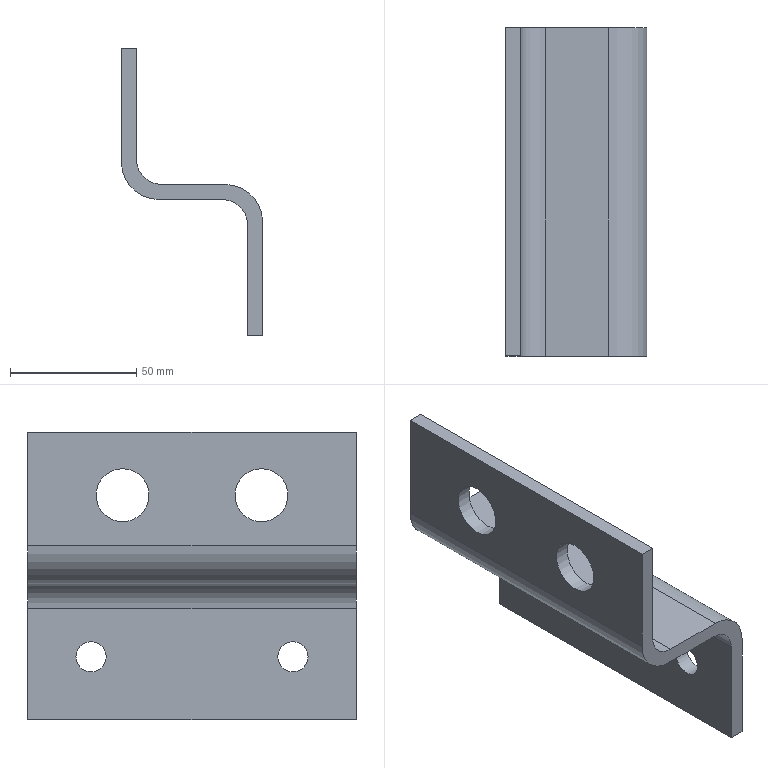Part | NX | features solid 2 | 1 solid | 18 faces | box 56 x 130 x 114 mm | volume 115432 mm3 | plane 10 | cylinder 8 | commonest cylinder face diameters 12 x2 20 x2 21 x2 30 x2
STEP:
#1=CARTESIAN_POINT('',(1315.,-200.,-620.));
#2=VERTEX_POINT('',#1);
#3=CARTESIAN_POINT('',(1321.,-200.,-620.));
#4=VERTEX_POINT('',#3);
#5=CARTESIAN_POINT('',(1325.,-200.,-620.));
#6=DIRECTION('',(-1.,0.,0.));
#7=VECTOR('',#6,1000.);
#8=LINE('',#5,#7);
#9=EDGE_CURVE('',#2,#4,#8,.F.);
#10=ORIENTED_EDGE('',*,*,#9,.T.);
#11=CARTESIAN_POINT('',(1321.,-330.,-620.));
#12=VERTEX_POINT('',#11);
#13=CARTESIAN_POINT('',(1321.,-130.,-620.));
#14=DIRECTION('',(0.,1.,0.));
#15=VECTOR('',#14,1000.);
#16=LINE('',#13,#15);
#17=EDGE_CURVE('',#4,#12,#16,.F.);
#18=ORIENTED_EDGE('',*,*,#17,.T.);
#19=CARTESIAN_POINT('',(1315.,-330.,-620.));
#20=VERTEX_POINT('',#19);
#21=CARTESIAN_POINT('',(1315.,-330.,-620.));
#22=DIRECTION('',(1.,0.,0.));
#23=VECTOR('',#22,1000.);
#24=LINE('',#21,#23);
#25=EDGE_CURVE('',#20,#12,#24,.T.);
#26=ORIENTED_EDGE('',*,*,#25,.F.);
#27=CARTESIAN_POINT('',(1315.,-130.,-620.));
#28=DIRECTION('',(0.,1.,0.));
#29=VECTOR('',#28,1000.);
#30=LINE('',#27,#29);
#31=EDGE_CURVE('',#2,#20,#30,.F.);
#32=ORIENTED_EDGE('',*,*,#31,.F.);
#33=EDGE_LOOP('',(#10,#18,#26,#32));
#34=FACE_BOUND('',#33,.T.);
#35=CARTESIAN_POINT('',(1325.,-130.,-620.));
#36=DIRECTION('',(0.,0.,-1.));
#37=DIRECTION('',(-1.,0.,0.));
#38=AXIS2_PLACEMENT_3D('',#35,#36,#37);
#39=PLANE('',#38);
#40=ADVANCED_FACE('',(#34),#39,.T.);
#41=CARTESIAN_POINT('',(1321.,-330.,-575.));
#42=VERTEX_POINT('',#41);
#43=CARTESIAN_POINT('',(1321.,-330.,-610.));
#44=DIRECTION('',(0.,0.,1.));
#45=VECTOR('',#44,1000.);
#46=LINE('',#43,#45);
#47=EDGE_CURVE('',#12,#42,#46,.T.);
#48=ORIENTED_EDGE('',*,*,#47,.T.);
#49=CARTESIAN_POINT('',(1306.,-330.,-560.));
#50=VERTEX_POINT('',#49);
#51=CARTESIAN_POINT('',(1306.,-330.,-575.));
#52=DIRECTION('',(0.,-1.,0.));
#53=DIRECTION('',(1.,0.,0.));
#54=AXIS2_PLACEMENT_3D('',#51,#52,#53);
#55=CIRCLE('',#54,15.);
#56=EDGE_CURVE('',#42,#50,#55,.T.);
#57=ORIENTED_EDGE('',*,*,#56,.T.);
#58=CARTESIAN_POINT('',(1281.,-330.,-560.));
#59=VERTEX_POINT('',#58);
#60=CARTESIAN_POINT('',(1315.,-330.,-560.));
#61=DIRECTION('',(-1.,0.,0.));
#62=VECTOR('',#61,1000.);
#63=LINE('',#60,#62);
#64=EDGE_CURVE('',#59,#50,#63,.F.);
#65=ORIENTED_EDGE('',*,*,#64,.F.);
#66=CARTESIAN_POINT('',(1271.,-330.,-550.));
#67=VERTEX_POINT('',#66);
#68=CARTESIAN_POINT('',(1281.,-330.,-550.));
#69=DIRECTION('',(0.,-1.,0.));
#70=DIRECTION('',(1.,0.,0.));
#71=AXIS2_PLACEMENT_3D('',#68,#69,#70);
#72=CIRCLE('',#71,10.);
#73=EDGE_CURVE('',#59,#67,#72,.F.);
#74=ORIENTED_EDGE('',*,*,#73,.T.);
#75=CARTESIAN_POINT('',(1271.,-330.,-506.));
#76=VERTEX_POINT('',#75);
#77=CARTESIAN_POINT('',(1271.,-330.,-504.5));
#78=DIRECTION('',(0.,0.,1.));
#79=VECTOR('',#78,1000.);
#80=LINE('',#77,#79);
#81=EDGE_CURVE('',#76,#67,#80,.F.);
#82=ORIENTED_EDGE('',*,*,#81,.F.);
#83=CARTESIAN_POINT('',(1265.,-330.,-506.));
#84=VERTEX_POINT('',#83);
#85=CARTESIAN_POINT('',(1267.,-330.,-506.));
#86=DIRECTION('',(-1.,0.,0.));
#87=VECTOR('',#86,1000.);
#88=LINE('',#85,#87);
#89=EDGE_CURVE('',#76,#84,#88,.T.);
#90=ORIENTED_EDGE('',*,*,#89,.T.);
#91=CARTESIAN_POINT('',(1265.,-330.,-551.));
#92=VERTEX_POINT('',#91);
#93=CARTESIAN_POINT('',(1265.,-330.,-555.5));
#94=DIRECTION('',(0.,0.,1.));
#95=VECTOR('',#94,1000.);
#96=LINE('',#93,#95);
#97=EDGE_CURVE('',#84,#92,#96,.F.);
#98=ORIENTED_EDGE('',*,*,#97,.T.);
#99=CARTESIAN_POINT('',(1280.,-330.,-566.));
#100=VERTEX_POINT('',#99);
#101=CARTESIAN_POINT('',(1280.,-330.,-551.));
#102=DIRECTION('',(0.,-1.,0.));
#103=DIRECTION('',(1.,0.,0.));
#104=AXIS2_PLACEMENT_3D('',#101,#102,#103);
#105=CIRCLE('',#104,15.);
#106=EDGE_CURVE('',#92,#100,#105,.T.);
#107=ORIENTED_EDGE('',*,*,#106,.T.);
#108=CARTESIAN_POINT('',(1305.,-330.,-566.));
#109=VERTEX_POINT('',#108);
#110=CARTESIAN_POINT('',(1271.,-330.,-566.));
#111=DIRECTION('',(-1.,0.,0.));
#112=VECTOR('',#111,1000.);
#113=LINE('',#110,#112);
#114=EDGE_CURVE('',#100,#109,#113,.F.);
#115=ORIENTED_EDGE('',*,*,#114,.T.);
#116=CARTESIAN_POINT('',(1315.,-330.,-576.));
#117=VERTEX_POINT('',#116);
#118=CARTESIAN_POINT('',(1305.,-330.,-576.));
#119=DIRECTION('',(0.,-1.,0.));
#120=DIRECTION('',(1.,0.,0.));
#121=AXIS2_PLACEMENT_3D('',#118,#119,#120);
#122=CIRCLE('',#121,10.);
#123=EDGE_CURVE('',#109,#117,#122,.F.);
#124=ORIENTED_EDGE('',*,*,#123,.T.);
#125=CARTESIAN_POINT('',(1315.,-330.,-610.));
#126=DIRECTION('',(0.,0.,1.));
#127=VECTOR('',#126,1000.);
#128=LINE('',#125,#127);
#129=EDGE_CURVE('',#20,#117,#128,.T.);
#130=ORIENTED_EDGE('',*,*,#129,.F.);
#131=ORIENTED_EDGE('',*,*,#25,.T.);
#132=EDGE_LOOP('',(#48,#57,#65,#74,#82,#90,#98,#107,#115,#124,#130,#131));
#133=FACE_BOUND('',#132,.T.);
#134=CARTESIAN_POINT('',(1315.,-330.,-610.));
#135=DIRECTION('',(0.,-1.,0.));
#136=DIRECTION('',(0.,0.,1.));
#137=AXIS2_PLACEMENT_3D('',#134,#135,#136);
#138=PLANE('',#137);
#139=ADVANCED_FACE('',(#133),#138,.T.);
#140=ORIENTED_EDGE('',*,*,#64,.T.);
#141=CARTESIAN_POINT('',(1306.,-200.,-560.));
#142=VERTEX_POINT('',#141);
#143=CARTESIAN_POINT('',(1306.,-200.,-560.));
#144=DIRECTION('',(0.,-1.,0.));
#145=VECTOR('',#144,1000.);
#146=LINE('',#143,#145);
#147=EDGE_CURVE('',#50,#142,#146,.F.);
#148=ORIENTED_EDGE('',*,*,#147,.T.);
#149=CARTESIAN_POINT('',(1281.,-200.,-560.));
#150=VERTEX_POINT('',#149);
#151=CARTESIAN_POINT('',(1315.,-200.,-560.));
#152=DIRECTION('',(-1.,0.,0.));
#153=VECTOR('',#152,1000.);
#154=LINE('',#151,#153);
#155=EDGE_CURVE('',#150,#142,#154,.F.);
#156=ORIENTED_EDGE('',*,*,#155,.F.);
#157=CARTESIAN_POINT('',(1281.,-200.,-560.));
#158=DIRECTION('',(0.,1.,0.));
#159=VECTOR('',#158,1000.);
#160=LINE('',#157,#159);
#161=EDGE_CURVE('',#150,#59,#160,.F.);
#162=ORIENTED_EDGE('',*,*,#161,.T.);
#163=EDGE_LOOP('',(#140,#148,#156,#162));
#164=FACE_BOUND('',#163,.T.);
#165=CARTESIAN_POINT('',(1315.,-200.,-560.));
#166=DIRECTION('',(0.,0.,-1.));
#167=DIRECTION('',(0.,-1.,0.));
#168=AXIS2_PLACEMENT_3D('',#165,#166,#167);
#169=PLANE('',#168);
#170=ADVANCED_FACE('',(#164),#169,.F.);
#171=ORIENTED_EDGE('',*,*,#155,.T.);
#172=CARTESIAN_POINT('',(1321.,-200.,-575.));
#173=VERTEX_POINT('',#172);
#174=CARTESIAN_POINT('',(1306.,-200.,-575.));
#175=DIRECTION('',(0.,-1.,0.));
#176=DIRECTION('',(1.,0.,0.));
#177=AXIS2_PLACEMENT_3D('',#174,#175,#176);
#178=CIRCLE('',#177,15.);
#179=EDGE_CURVE('',#142,#173,#178,.F.);
#180=ORIENTED_EDGE('',*,*,#179,.T.);
#181=CARTESIAN_POINT('',(1321.,-200.,-610.));
#182=DIRECTION('',(0.,0.,1.));
#183=VECTOR('',#182,1000.);
#184=LINE('',#181,#183);
#185=EDGE_CURVE('',#4,#173,#184,.T.);
#186=ORIENTED_EDGE('',*,*,#185,.F.);
#187=ORIENTED_EDGE('',*,*,#9,.F.);
#188=CARTESIAN_POINT('',(1315.,-200.,-576.));
#189=VERTEX_POINT('',#188);
#190=CARTESIAN_POINT('',(1315.,-200.,-610.));
#191=DIRECTION('',(0.,0.,1.));
#192=VECTOR('',#191,1000.);
#193=LINE('',#190,#192);
#194=EDGE_CURVE('',#2,#189,#193,.T.);
#195=ORIENTED_EDGE('',*,*,#194,.T.);
#196=CARTESIAN_POINT('',(1305.,-200.,-566.));
#197=VERTEX_POINT('',#196);
#198=CARTESIAN_POINT('',(1305.,-200.,-576.));
#199=DIRECTION('',(0.,-1.,0.));
#200=DIRECTION('',(1.,0.,0.));
#201=AXIS2_PLACEMENT_3D('',#198,#199,#200);
#202=CIRCLE('',#201,10.);
#203=EDGE_CURVE('',#189,#197,#202,.T.);
#204=ORIENTED_EDGE('',*,*,#203,.T.);
#205=CARTESIAN_POINT('',(1280.,-200.,-566.));
#206=VERTEX_POINT('',#205);
#207=CARTESIAN_POINT('',(1271.,-200.,-566.));
#208=DIRECTION('',(-1.,0.,0.));
#209=VECTOR('',#208,1000.);
#210=LINE('',#207,#209);
#211=EDGE_CURVE('',#206,#197,#210,.F.);
#212=ORIENTED_EDGE('',*,*,#211,.F.);
#213=CARTESIAN_POINT('',(1265.,-200.,-551.));
#214=VERTEX_POINT('',#213);
#215=CARTESIAN_POINT('',(1280.,-200.,-551.));
#216=DIRECTION('',(0.,-1.,0.));
#217=DIRECTION('',(1.,0.,0.));
#218=AXIS2_PLACEMENT_3D('',#215,#216,#217);
#219=CIRCLE('',#218,15.);
#220=EDGE_CURVE('',#206,#214,#219,.F.);
#221=ORIENTED_EDGE('',*,*,#220,.T.);
#222=CARTESIAN_POINT('',(1265.,-200.,-506.));
#223=VERTEX_POINT('',#222);
#224=CARTESIAN_POINT('',(1265.,-200.,-516.));
#225=DIRECTION('',(0.,0.,-1.));
#226=VECTOR('',#225,1000.);
#227=LINE('',#224,#226);
#228=EDGE_CURVE('',#223,#214,#227,.T.);
#229=ORIENTED_EDGE('',*,*,#228,.F.);
#230=CARTESIAN_POINT('',(1271.,-200.,-506.));
#231=VERTEX_POINT('',#230);
#232=CARTESIAN_POINT('',(1267.,-200.,-506.));
#233=DIRECTION('',(1.,0.,0.));
#234=VECTOR('',#233,1000.);
#235=LINE('',#232,#234);
#236=EDGE_CURVE('',#231,#223,#235,.F.);
#237=ORIENTED_EDGE('',*,*,#236,.F.);
#238=CARTESIAN_POINT('',(1271.,-200.,-550.));
#239=VERTEX_POINT('',#238);
#240=CARTESIAN_POINT('',(1271.,-200.,-516.));
#241=DIRECTION('',(0.,0.,-1.));
#242=VECTOR('',#241,1000.);
#243=LINE('',#240,#242);
#244=EDGE_CURVE('',#231,#239,#243,.T.);
#245=ORIENTED_EDGE('',*,*,#244,.T.);
#246=CARTESIAN_POINT('',(1281.,-200.,-550.));
#247=DIRECTION('',(0.,-1.,0.));
#248=DIRECTION('',(1.,0.,0.));
#249=AXIS2_PLACEMENT_3D('',#246,#247,#248);
#250=CIRCLE('',#249,10.);
#251=EDGE_CURVE('',#239,#150,#250,.T.);
#252=ORIENTED_EDGE('',*,*,#251,.T.);
#253=EDGE_LOOP('',(#171,#180,#186,#187,#195,#204,#212,#221,#229,#237,#245,#252));
#254=FACE_BOUND('',#253,.T.);
#255=CARTESIAN_POINT('',(1315.,-200.,-610.));
#256=DIRECTION('',(0.,-1.,0.));
#257=DIRECTION('',(0.,0.,1.));
#258=AXIS2_PLACEMENT_3D('',#255,#256,#257);
#259=PLANE('',#258);
#260=ADVANCED_FACE('',(#254),#259,.F.);
#261=CARTESIAN_POINT('',(1321.,-231.,-595.));
#262=VERTEX_POINT('',#261);
#263=CARTESIAN_POINT('',(1321.,-225.,-595.));
#264=DIRECTION('',(-1.,0.,0.));
#265=DIRECTION('',(0.,-1.,0.));
#266=AXIS2_PLACEMENT_3D('',#263,#264,#265);
#267=CIRCLE('',#266,6.);
#268=EDGE_CURVE('',#262,#262,#267,.T.);
#269=ORIENTED_EDGE('',*,*,#268,.T.);
#270=EDGE_LOOP('',(#269));
#271=FACE_BOUND('',#270,.T.);
#272=CARTESIAN_POINT('',(1321.,-311.,-595.));
#273=VERTEX_POINT('',#272);
#274=CARTESIAN_POINT('',(1321.,-305.,-595.));
#275=DIRECTION('',(-1.,0.,0.));
#276=DIRECTION('',(0.,-1.,0.));
#277=AXIS2_PLACEMENT_3D('',#274,#275,#276);
#278=CIRCLE('',#277,6.);
#279=EDGE_CURVE('',#273,#273,#278,.T.);
#280=ORIENTED_EDGE('',*,*,#279,.T.);
#281=EDGE_LOOP('',(#280));
#282=FACE_BOUND('',#281,.T.);
#283=ORIENTED_EDGE('',*,*,#185,.T.);
#284=CARTESIAN_POINT('',(1321.,-200.,-575.));
#285=DIRECTION('',(0.,-1.,0.));
#286=VECTOR('',#285,1000.);
#287=LINE('',#284,#286);
#288=EDGE_CURVE('',#173,#42,#287,.T.);
#289=ORIENTED_EDGE('',*,*,#288,.T.);
#290=ORIENTED_EDGE('',*,*,#47,.F.);
#291=ORIENTED_EDGE('',*,*,#17,.F.);
#292=EDGE_LOOP('',(#283,#289,#290,#291));
#293=FACE_BOUND('',#292,.T.);
#294=CARTESIAN_POINT('',(1321.,-200.,-610.));
#295=DIRECTION('',(-1.,0.,0.));
#296=DIRECTION('',(0.,-1.,0.));
#297=AXIS2_PLACEMENT_3D('',#294,#295,#296);
#298=PLANE('',#297);
#299=ADVANCED_FACE('',(#271,#282,#293),#298,.F.);
#300=CARTESIAN_POINT('',(1315.,-231.,-595.));
#301=VERTEX_POINT('',#300);
#302=CARTESIAN_POINT('',(1315.,-225.,-595.));
#303=DIRECTION('',(-1.,0.,0.));
#304=DIRECTION('',(0.,-1.,0.));
#305=AXIS2_PLACEMENT_3D('',#302,#303,#304);
#306=CIRCLE('',#305,6.);
#307=EDGE_CURVE('',#301,#301,#306,.T.);
#308=ORIENTED_EDGE('',*,*,#307,.F.);
#309=EDGE_LOOP('',(#308));
#310=FACE_BOUND('',#309,.T.);
#311=CARTESIAN_POINT('',(1315.,-311.,-595.));
#312=VERTEX_POINT('',#311);
#313=CARTESIAN_POINT('',(1315.,-305.,-595.));
#314=DIRECTION('',(-1.,0.,0.));
#315=DIRECTION('',(0.,-1.,0.));
#316=AXIS2_PLACEMENT_3D('',#313,#314,#315);
#317=CIRCLE('',#316,6.);
#318=EDGE_CURVE('',#312,#312,#317,.T.);
#319=ORIENTED_EDGE('',*,*,#318,.F.);
#320=EDGE_LOOP('',(#319));
#321=FACE_BOUND('',#320,.T.);
#322=ORIENTED_EDGE('',*,*,#129,.T.);
#323=CARTESIAN_POINT('',(1315.,-200.,-576.));
#324=DIRECTION('',(0.,-1.,0.));
#325=VECTOR('',#324,1000.);
#326=LINE('',#323,#325);
#327=EDGE_CURVE('',#117,#189,#326,.F.);
#328=ORIENTED_EDGE('',*,*,#327,.T.);
#329=ORIENTED_EDGE('',*,*,#194,.F.);
#330=ORIENTED_EDGE('',*,*,#31,.T.);
#331=EDGE_LOOP('',(#322,#328,#329,#330));
#332=FACE_BOUND('',#331,.T.);
#333=CARTESIAN_POINT('',(1315.,-200.,-610.));
#334=DIRECTION('',(-1.,0.,0.));
#335=DIRECTION('',(0.,-1.,0.));
#336=AXIS2_PLACEMENT_3D('',#333,#334,#335);
#337=PLANE('',#336);
#338=ADVANCED_FACE('',(#310,#321,#332),#337,.T.);
#339=ORIENTED_EDGE('',*,*,#211,.T.);
#340=CARTESIAN_POINT('',(1305.,-200.,-566.));
#341=DIRECTION('',(0.,-1.,0.));
#342=VECTOR('',#341,1000.);
#343=LINE('',#340,#342);
#344=EDGE_CURVE('',#197,#109,#343,.T.);
#345=ORIENTED_EDGE('',*,*,#344,.T.);
#346=ORIENTED_EDGE('',*,*,#114,.F.);
#347=CARTESIAN_POINT('',(1280.,-200.,-566.));
#348=DIRECTION('',(0.,1.,0.));
#349=VECTOR('',#348,1000.);
#350=LINE('',#347,#349);
#351=EDGE_CURVE('',#100,#206,#350,.T.);
#352=ORIENTED_EDGE('',*,*,#351,.T.);
#353=EDGE_LOOP('',(#339,#345,#346,#352));
#354=FACE_BOUND('',#353,.T.);
#355=CARTESIAN_POINT('',(1271.,-200.,-566.));
#356=DIRECTION('',(0.,0.,1.));
#357=DIRECTION('',(0.,-1.,0.));
#358=AXIS2_PLACEMENT_3D('',#355,#356,#357);
#359=PLANE('',#358);
#360=ADVANCED_FACE('',(#354),#359,.F.);
#361=CARTESIAN_POINT('',(1271.,-292.5,-520.5));
#362=VERTEX_POINT('',#361);
#363=CARTESIAN_POINT('',(1271.,-292.5,-531.));
#364=DIRECTION('',(-1.,0.,0.));
#365=DIRECTION('',(0.,0.,1.));
#366=AXIS2_PLACEMENT_3D('',#363,#364,#365);
#367=CIRCLE('',#366,10.5);
#368=EDGE_CURVE('',#362,#362,#367,.T.);
#369=ORIENTED_EDGE('',*,*,#368,.T.);
#370=EDGE_LOOP('',(#369));
#371=FACE_BOUND('',#370,.T.);
#372=CARTESIAN_POINT('',(1271.,-237.5,-520.5));
#373=VERTEX_POINT('',#372);
#374=CARTESIAN_POINT('',(1271.,-237.5,-531.));
#375=DIRECTION('',(-1.,0.,0.));
#376=DIRECTION('',(0.,0.,1.));
#377=AXIS2_PLACEMENT_3D('',#374,#375,#376);
#378=CIRCLE('',#377,10.5);
#379=EDGE_CURVE('',#373,#373,#378,.F.);
#380=ORIENTED_EDGE('',*,*,#379,.F.);
#381=EDGE_LOOP('',(#380));
#382=FACE_BOUND('',#381,.T.);
#383=ORIENTED_EDGE('',*,*,#81,.T.);
#384=CARTESIAN_POINT('',(1271.,-222.778,-550.));
#385=DIRECTION('',(0.,-1.,0.));
#386=VECTOR('',#385,1000.);
#387=LINE('',#384,#386);
#388=EDGE_CURVE('',#67,#239,#387,.F.);
#389=ORIENTED_EDGE('',*,*,#388,.T.);
#390=ORIENTED_EDGE('',*,*,#244,.F.);
#391=CARTESIAN_POINT('',(1271.,-222.778,-506.));
#392=DIRECTION('',(0.,1.,0.));
#393=VECTOR('',#392,1000.);
#394=LINE('',#391,#393);
#395=EDGE_CURVE('',#231,#76,#394,.F.);
#396=ORIENTED_EDGE('',*,*,#395,.T.);
#397=EDGE_LOOP('',(#383,#389,#390,#396));
#398=FACE_BOUND('',#397,.T.);
#399=CARTESIAN_POINT('',(1271.,-222.778,-504.5));
#400=DIRECTION('',(-1.,0.,0.));
#401=DIRECTION('',(0.,-1.,0.));
#402=AXIS2_PLACEMENT_3D('',#399,#400,#401);
#403=PLANE('',#402);
#404=ADVANCED_FACE('',(#371,#382,#398),#403,.F.);
#405=ORIENTED_EDGE('',*,*,#89,.F.);
#406=ORIENTED_EDGE('',*,*,#395,.F.);
#407=ORIENTED_EDGE('',*,*,#236,.T.);
#408=CARTESIAN_POINT('',(1265.,-222.778,-506.));
#409=DIRECTION('',(0.,1.,0.));
#410=VECTOR('',#409,1000.);
#411=LINE('',#408,#410);
#412=EDGE_CURVE('',#223,#84,#411,.F.);
#413=ORIENTED_EDGE('',*,*,#412,.T.);
#414=EDGE_LOOP('',(#405,#406,#407,#413));
#415=FACE_BOUND('',#414,.T.);
#416=CARTESIAN_POINT('',(1267.,-200.,-506.));
#417=DIRECTION('',(0.,0.,1.));
#418=DIRECTION('',(0.,-1.,0.));
#419=AXIS2_PLACEMENT_3D('',#416,#417,#418);
#420=PLANE('',#419);
#421=ADVANCED_FACE('',(#415),#420,.T.);
#422=CARTESIAN_POINT('',(1265.,-292.5,-520.5));
#423=VERTEX_POINT('',#422);
#424=CARTESIAN_POINT('',(1265.,-292.5,-531.));
#425=DIRECTION('',(-1.,0.,0.));
#426=DIRECTION('',(0.,0.,1.));
#427=AXIS2_PLACEMENT_3D('',#424,#425,#426);
#428=CIRCLE('',#427,10.5);
#429=EDGE_CURVE('',#423,#423,#428,.F.);
#430=ORIENTED_EDGE('',*,*,#429,.T.);
#431=EDGE_LOOP('',(#430));
#432=FACE_BOUND('',#431,.T.);
#433=CARTESIAN_POINT('',(1265.,-237.5,-541.5));
#434=VERTEX_POINT('',#433);
#435=CARTESIAN_POINT('',(1265.,-237.5,-531.));
#436=DIRECTION('',(1.,0.,0.));
#437=DIRECTION('',(0.,0.,-1.));
#438=AXIS2_PLACEMENT_3D('',#435,#436,#437);
#439=CIRCLE('',#438,10.5);
#440=EDGE_CURVE('',#434,#434,#439,.T.);
#441=ORIENTED_EDGE('',*,*,#440,.T.);
#442=EDGE_LOOP('',(#441));
#443=FACE_BOUND('',#442,.T.);
#444=ORIENTED_EDGE('',*,*,#228,.T.);
#445=CARTESIAN_POINT('',(1265.,-222.778,-551.));
#446=DIRECTION('',(0.,-1.,0.));
#447=VECTOR('',#446,1000.);
#448=LINE('',#445,#447);
#449=EDGE_CURVE('',#214,#92,#448,.T.);
#450=ORIENTED_EDGE('',*,*,#449,.T.);
#451=ORIENTED_EDGE('',*,*,#97,.F.);
#452=ORIENTED_EDGE('',*,*,#412,.F.);
#453=EDGE_LOOP('',(#444,#450,#451,#452));
#454=FACE_BOUND('',#453,.T.);
#455=CARTESIAN_POINT('',(1265.,-222.778,-555.5));
#456=DIRECTION('',(-1.,0.,0.));
#457=DIRECTION('',(0.,-1.,0.));
#458=AXIS2_PLACEMENT_3D('',#455,#456,#457);
#459=PLANE('',#458);
#460=ADVANCED_FACE('',(#432,#443,#454),#459,.T.);
#461=ORIENTED_EDGE('',*,*,#251,.F.);
#462=ORIENTED_EDGE('',*,*,#388,.F.);
#463=ORIENTED_EDGE('',*,*,#73,.F.);
#464=ORIENTED_EDGE('',*,*,#161,.F.);
#465=EDGE_LOOP('',(#461,#462,#463,#464));
#466=FACE_BOUND('',#465,.T.);
#467=CARTESIAN_POINT('',(1281.,-200.,-550.));
#468=DIRECTION('',(0.,1.,0.));
#469=DIRECTION('',(0.,0.,1.));
#470=AXIS2_PLACEMENT_3D('',#467,#468,#469);
#471=CYLINDRICAL_SURFACE('',#470,10.);
#472=ADVANCED_FACE('',(#466),#471,.F.);
#473=ORIENTED_EDGE('',*,*,#220,.F.);
#474=ORIENTED_EDGE('',*,*,#351,.F.);
#475=ORIENTED_EDGE('',*,*,#106,.F.);
#476=ORIENTED_EDGE('',*,*,#449,.F.);
#477=EDGE_LOOP('',(#473,#474,#475,#476));
#478=FACE_BOUND('',#477,.T.);
#479=CARTESIAN_POINT('',(1280.,-222.778,-551.));
#480=DIRECTION('',(0.,1.,0.));
#481=DIRECTION('',(0.,0.,1.));
#482=AXIS2_PLACEMENT_3D('',#479,#480,#481);
#483=CYLINDRICAL_SURFACE('',#482,15.);
#484=ADVANCED_FACE('',(#478),#483,.T.);
#485=ORIENTED_EDGE('',*,*,#179,.F.);
#486=ORIENTED_EDGE('',*,*,#147,.F.);
#487=ORIENTED_EDGE('',*,*,#56,.F.);
#488=ORIENTED_EDGE('',*,*,#288,.F.);
#489=EDGE_LOOP('',(#485,#486,#487,#488));
#490=FACE_BOUND('',#489,.T.);
#491=CARTESIAN_POINT('',(1306.,-200.,-575.));
#492=DIRECTION('',(0.,-1.,0.));
#493=DIRECTION('',(1.,0.,0.));
#494=AXIS2_PLACEMENT_3D('',#491,#492,#493);
#495=CYLINDRICAL_SURFACE('',#494,15.);
#496=ADVANCED_FACE('',(#490),#495,.T.);
#497=ORIENTED_EDGE('',*,*,#203,.F.);
#498=ORIENTED_EDGE('',*,*,#327,.F.);
#499=ORIENTED_EDGE('',*,*,#123,.F.);
#500=ORIENTED_EDGE('',*,*,#344,.F.);
#501=EDGE_LOOP('',(#497,#498,#499,#500));
#502=FACE_BOUND('',#501,.T.);
#503=CARTESIAN_POINT('',(1305.,-200.,-576.));
#504=DIRECTION('',(0.,-1.,0.));
#505=DIRECTION('',(1.,0.,0.));
#506=AXIS2_PLACEMENT_3D('',#503,#504,#505);
#507=CYLINDRICAL_SURFACE('',#506,10.);
#508=ADVANCED_FACE('',(#502),#507,.F.);
#509=ORIENTED_EDGE('',*,*,#318,.T.);
#510=EDGE_LOOP('',(#509));
#511=FACE_BOUND('',#510,.T.);
#512=ORIENTED_EDGE('',*,*,#279,.F.);
#513=EDGE_LOOP('',(#512));
#514=FACE_BOUND('',#513,.T.);
#515=CARTESIAN_POINT('',(1321.,-305.,-595.));
#516=DIRECTION('',(-1.,0.,0.));
#517=DIRECTION('',(0.,-1.,0.));
#518=AXIS2_PLACEMENT_3D('',#515,#516,#517);
#519=CYLINDRICAL_SURFACE('',#518,6.);
#520=ADVANCED_FACE('',(#511,#514),#519,.F.);
#521=ORIENTED_EDGE('',*,*,#307,.T.);
#522=EDGE_LOOP('',(#521));
#523=FACE_BOUND('',#522,.T.);
#524=ORIENTED_EDGE('',*,*,#268,.F.);
#525=EDGE_LOOP('',(#524));
#526=FACE_BOUND('',#525,.T.);
#527=CARTESIAN_POINT('',(1321.,-225.,-595.));
#528=DIRECTION('',(-1.,0.,0.));
#529=DIRECTION('',(0.,-1.,0.));
#530=AXIS2_PLACEMENT_3D('',#527,#528,#529);
#531=CYLINDRICAL_SURFACE('',#530,6.);
#532=ADVANCED_FACE('',(#523,#526),#531,.F.);
#533=ORIENTED_EDGE('',*,*,#379,.T.);
#534=EDGE_LOOP('',(#533));
#535=FACE_BOUND('',#534,.T.);
#536=ORIENTED_EDGE('',*,*,#440,.F.);
#537=EDGE_LOOP('',(#536));
#538=FACE_BOUND('',#537,.T.);
#539=CARTESIAN_POINT('',(1265.,-237.5,-531.));
#540=DIRECTION('',(1.,0.,0.));
#541=DIRECTION('',(0.,0.,-1.));
#542=AXIS2_PLACEMENT_3D('',#539,#540,#541);
#543=CYLINDRICAL_SURFACE('',#542,10.5);
#544=ADVANCED_FACE('',(#535,#538),#543,.F.);
#545=ORIENTED_EDGE('',*,*,#368,.F.);
#546=EDGE_LOOP('',(#545));
#547=FACE_BOUND('',#546,.T.);
#548=ORIENTED_EDGE('',*,*,#429,.F.);
#549=EDGE_LOOP('',(#548));
#550=FACE_BOUND('',#549,.T.);
#551=CARTESIAN_POINT('',(1271.,-292.5,-531.));
#552=DIRECTION('',(-1.,0.,0.));
#553=DIRECTION('',(0.,0.,1.));
#554=AXIS2_PLACEMENT_3D('',#551,#552,#553);
#555=CYLINDRICAL_SURFACE('',#554,10.5);
#556=ADVANCED_FACE('',(#547,#550),#555,.F.);
#557=CLOSED_SHELL('',(#40,#139,#170,#260,#299,#338,#360,#404,#421,#460,#472,#484,#496,#508,#520,#532,#544,#556));
#558=MANIFOLD_SOLID_BREP('',#557);
#559=(LENGTH_UNIT()NAMED_UNIT(*)SI_UNIT(.MILLI.,.METRE.));
#560=UNCERTAINTY_MEASURE_WITH_UNIT(LENGTH_MEASURE(0.00001),#559,'','');
#561=(NAMED_UNIT(*)PLANE_ANGLE_UNIT()SI_UNIT($,.RADIAN.));
#562=(NAMED_UNIT(*)SI_UNIT($,.STERADIAN.)SOLID_ANGLE_UNIT());
#563=(GEOMETRIC_REPRESENTATION_CONTEXT(3)GLOBAL_UNCERTAINTY_ASSIGNED_CONTEXT((#560))GLOBAL_UNIT_ASSIGNED_CONTEXT((#559,#561,#562))REPRESENTATION_CONTEXT('',''));
#564=ADVANCED_BREP_SHAPE_REPRESENTATION('',(#558),#563);